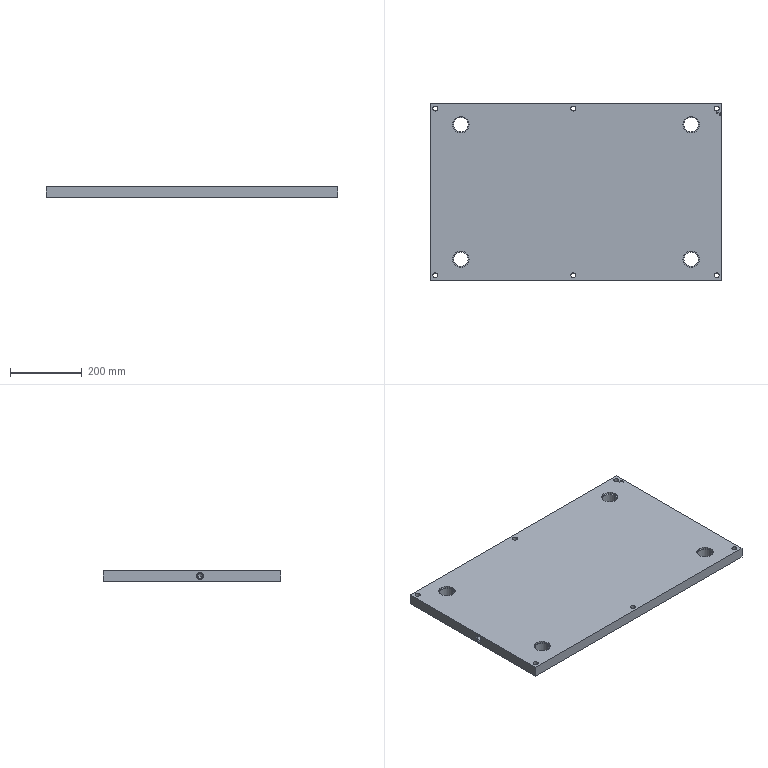Part | Creo | 1 solid | 75 faces | box 815 x 496 x 30 mm | volume 11917147 mm3 | cylinder 44 | plane 23 | cone 8 | commonest cylinder face diameters 14 x16 20 x12 40 x8 46 x8